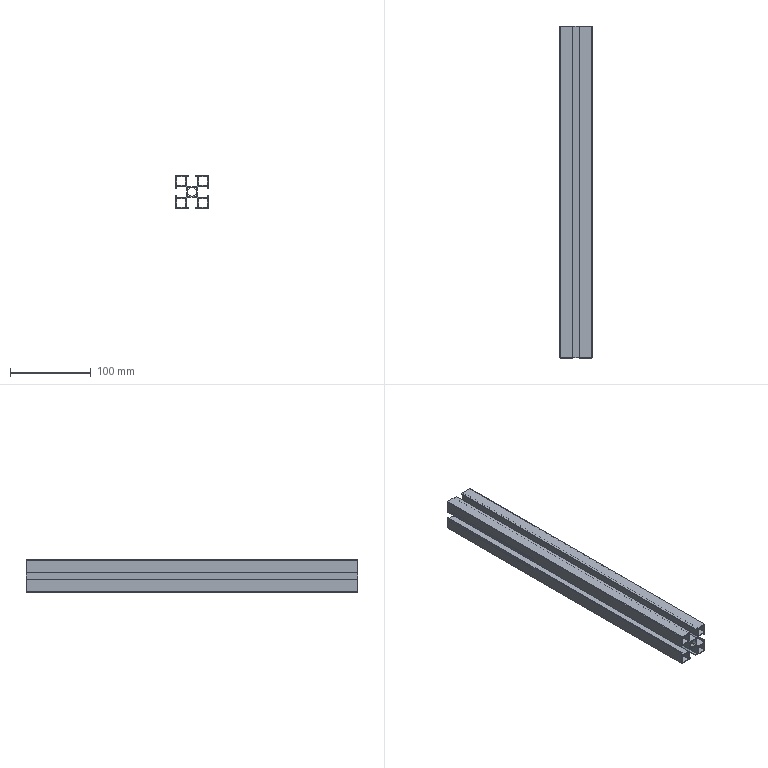Part | SolidWorks | features MirrorPattern 2, Extrusion 1 | 1 solid | 85 faces | box 40 x 410 x 40 mm | volume 106924 mm3 | plane 70 | cylinder 15 | commonest cylinder face diameters 2 x6 10.6 x5 1 x4